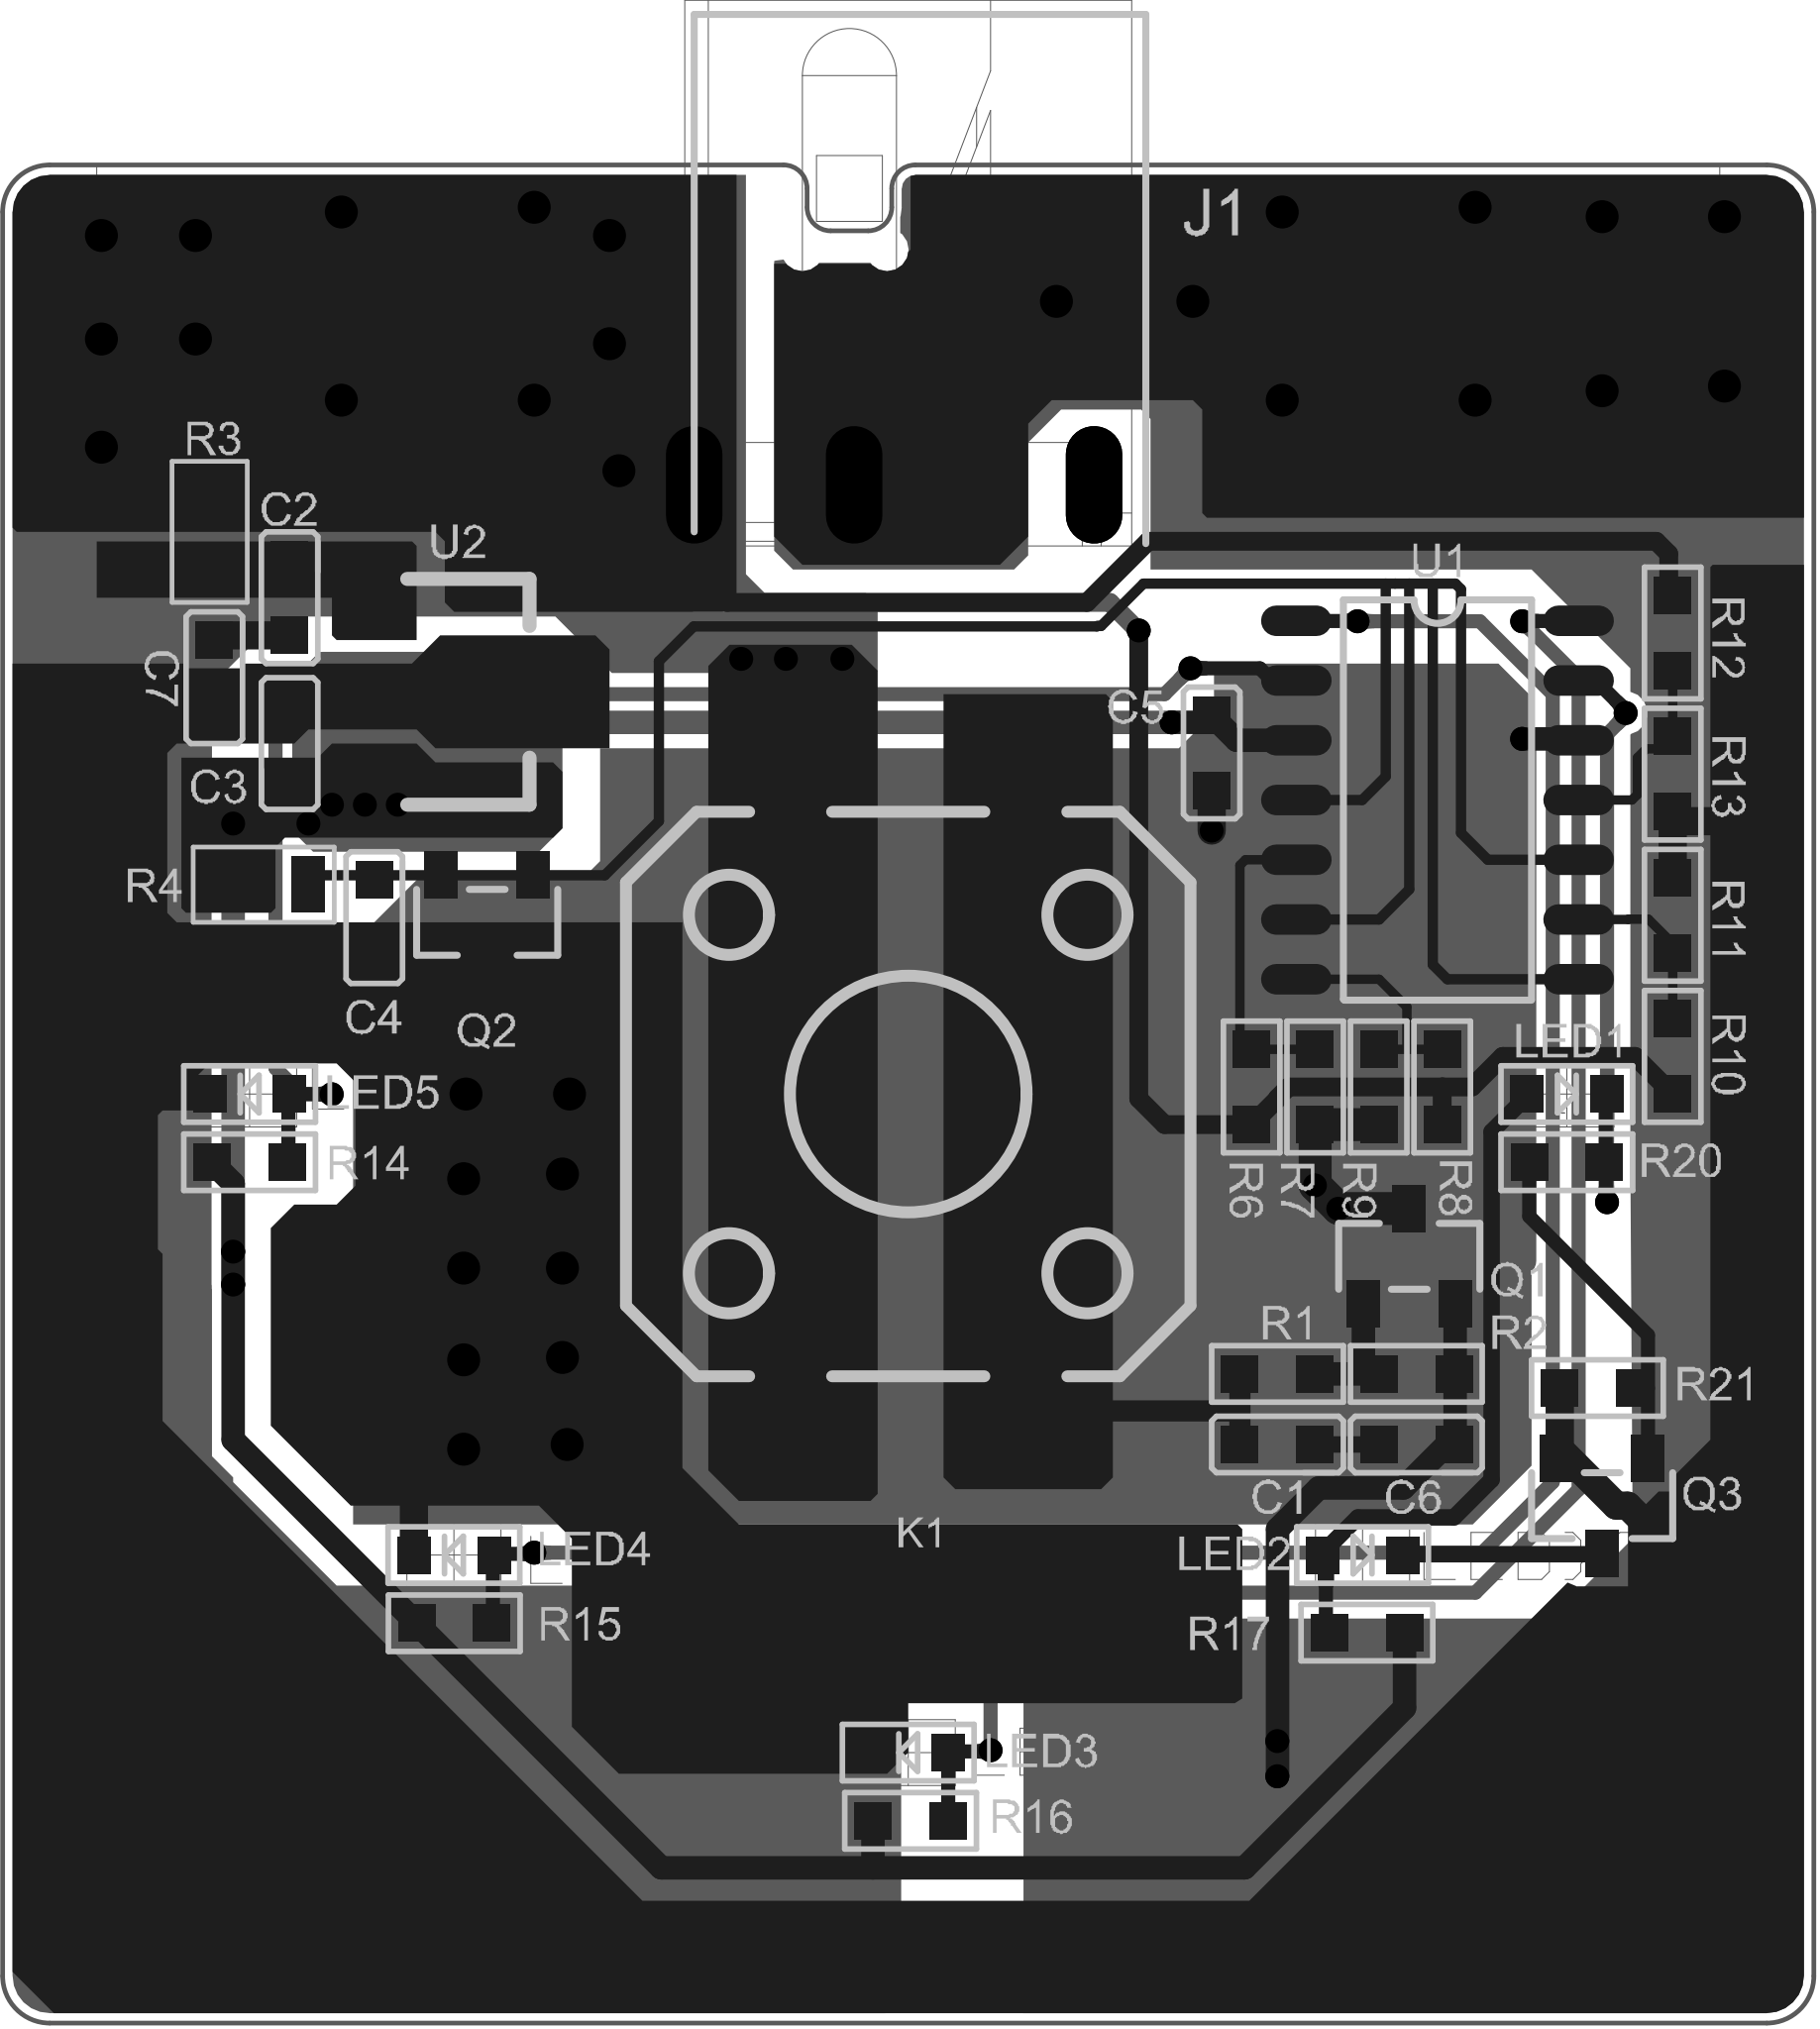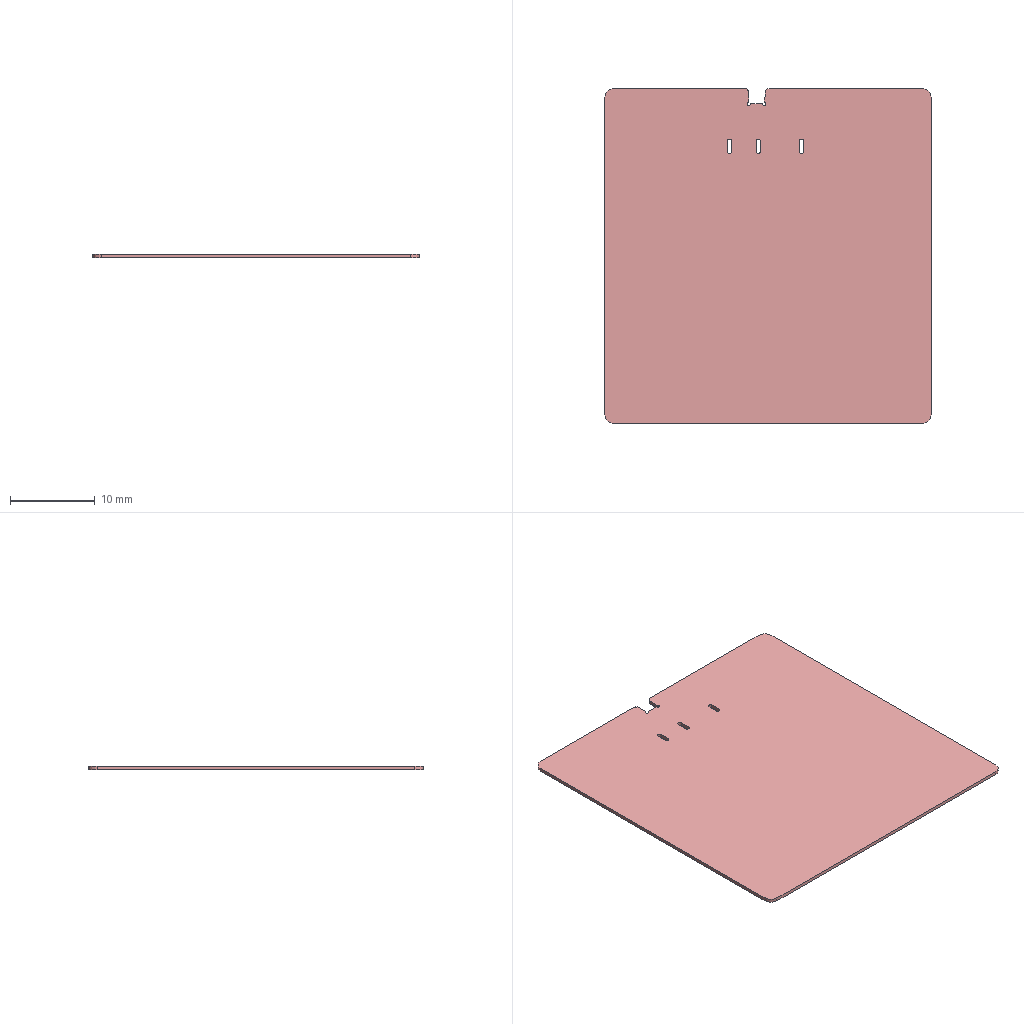Circuit board layout | Altium Designer | box 38.5 x 39.5 x 0.4 mm
Layer stack:
# Altium Designer layer stack of  (unit mm; dielectric type: 0 none, 1 core, 2 prepreg, 3 surface material)
index,name,kind,layer,copper_thickness_mm,dielectric_type,dielectric_thickness_mm,dielectric_material,dielectric_constant
0,Top Paste,other,,,,,,
1,Top Overlay,other,,,,,,
2,Top Solder,dielectric,,,3,0.0102,Solder Resist,3.5
3,Top Layer,copper,Top Layer,0.0356,,,,
4,Dielectric 1,dielectric,,,0,0.32,FR-4,4.8
5,Bottom Layer,copper,Bottom Layer,0.0356,,,,
6,Bottom Solder,dielectric,,,3,0.0102,Solder Resist,3.5
7,Bottom Overlay,other,,,,,,
8,Bottom Paste,other,,,,,,
# drill layer pairs: low layer,high layer
drill_pair,Top Layer,Bottom Layer
Part placement:
Designator,Comment,Layer,Footprint,Center-X(mm),Center-Y(mm),Rotation
U1,LM339,TopLayer,SOP14L,29.5,-13.5,0
K1,SW-PB,TopLayer,SW-SMD_4P-L12.0-W12.0-P5.00-LS15.2,18.25,-19.75,270
J1,DC-044/2.0芯卧插-耐高温260度,TopLayer,DC-044,17.95,-6.8,0
U2,DS8604,TopLayer,SOT-89-3,8.25,-11.2,270
R21,1M,TopLayer,R0603A,32.9,-26,0
R20,100K,TopLayer,R0603A,32.25,-21.2,0
R17,1K,TopLayer,R0603A,28,-31.2,180
R16,1K,TopLayer,R0603A,18.3,-35.2,0
R15,1K,TopLayer,R0603A,8.6,-31,0
R14,1K,TopLayer,R0603A,4.25,-21.2,0
R13,10K 1%,TopLayer,R0603A,34.5,-12.95,90
R12,120K,TopLayer,R0603A,34.5,-9.95,90
R11,10K 1%,TopLayer,R0603A,34.5,-15.95,270
R10,128.4K,TopLayer,R0603A,34.5,-18.95,270
R9,10K 1%,TopLayer,R0603A,28.25,-19.6,90
R8,136.4K,TopLayer,R0603A,29.6,-19.6,270
R7,10K 1%,TopLayer,R0603A,26.9,-19.6,90
R6,145.2K,TopLayer,R0603A,25.55,-19.6,270
R4,2K,TopLayer,R0805A,4.55,-15.3,180
R3,100R,TopLayer,R0805A,3.4,-7.8,90
R2,1M,TopLayer,R0603A,29.05,-25.7,0
R1,3M,TopLayer,R0603A,26.1,-25.7,0
Q3,2N7002,TopLayer,SOT23-3,33,-28.508,180
Q2,TL431_23,TopLayer,SOT23-3,9.3,-16.108,180
Q1,2N7002K,TopLayer,SOT23-3,28.9,-23.192,0
LED5,Green,TopLayer,LED0603A,4.25,-19.75,0
LED4,Green,TopLayer,LED0603A,8.593,-29.55,0
LED3,Green,TopLayer,LED0603A,18.25,-33.75,0
LED2,Green,TopLayer,LED0603A,27.907,-29.55,180
LED1,Green,TopLayer,LED0603A,32.25,-19.75,180
C7,1uF/50V,TopLayer,C0603A,3.5,-10.9,90
C6,1uF/50V,TopLayer,C0603A,29.05,-27.2,0
C5,1uF,TopLayer,C0603A,24.7,-12.5,90
C4,1uF,TopLayer,C0603A,6.9,-16,90
C3,1uF/50V,TopLayer,C0603A,5.1,-12.3,270
C2,1uF/50V,TopLayer,C0603A,5.1,-9.2,90
C1,1uF/50V,TopLayer,C0603A,26.1,-27.2,0
Pad and via stacks:
# Altium Designer via and pad stacks of  (unit mm). Each distinct definition once, with the count of objects using it.
# via: kind,start_layer,end_layer,hole_mm,diameter_mm,mode(0 simple;1 top-mid-bottom;2 full stack),diameter_per_layer,count,example_net
# pad: kind,layer,hole_mm,hole_type(0 round;1 square;2 slot),plating,top_size,top_shape(1 round;2 rect;3 octagon;9 rounded rect),mid_size,bottom_size,mode,footprint,size_per_layer,count,example
pad,Bottom Layer,0,0,plated,4x4,2,4x4,4x4,0,,,4,19
pad,Top Layer,0,0,plated,0.7x0.8,2,0.7x0.8,0.7x0.8,0,LED0603A,,10,LED2.2
pad,Top Layer,0,0,plated,0.8x0.8,2,0.8x0.8,0.8x0.8,0,R0603A,,32,R6.1
pad,Top Layer,0,0,plated,2.64x1.4,2,2.64x1.4,2.64x1.4,0,SW-SMD_4P-L12.0-W12.0-P5.00-LS15.2,,4,K1.1
pad,Top Layer,0,0,plated,0.7x1,2,0.7x1,0.7x1,0,SOT23-3,,9,Q1.1
pad,Top Layer,0,0,plated,0.8x0.8,2,0.8x0.8,0.8x0.8,0,C0603A,,14,C4.2
pad,Top Layer,0,0,plated,1x1,1,1x1,1x1,0,,,2,21
pad,Top Layer,0,2,plated,0.65x1.5,1,0.65x1.5,0.65x1.5,0,SOP14L,,14,U1.10
pad,Top Layer,0,0,plated,0.7x1.2,2,0.7x1.2,0.7x1.2,0,R0805A,,4,R4.2
pad,Top Layer,0,2,plated,1.5x0.65,2,1.5x0.65,1.5x0.65,0,SOT-89-3,,3,U2.1
pad,Top Layer,0,2,plated,2x3.8,1,2x3.8,2x3.8,0,SOT-89-3,,1,U2.2
pad,Multi-Layer,0.5,2,plated,2.5x1.2,1,2.5x1.2,2.5x1.2,0,DC-044,,3,J1.1
via,Top Layer,Bottom Layer,0.3048,0.508,0,,26,P+
via,Top Layer,Bottom Layer,0.5,0.7,0,,32,GND
Copper pours:
name,layer,net,type(0 solid;1 hatched;2 none)
NONET_L02_P-001,Bottom Layer,GND,0
NONET_L02_P-001,Bottom Layer,P-,0
NONET_L02_P-001,Bottom Layer,5V,0
NONET_L02_P-001,Bottom Layer,P+,0
NONET_L02_P-001,Top Layer,GND,0
NONET_L02_P-001,Top Layer,P+,0
NONET_L02_P-001,Top Layer,NetC1_1,0
NONET_L02_P-001,Top Layer,P-,0
NONET_L02_P-001,Top Layer,NetC2_2,0
NONET_L02_P-001,Top Layer,5V,0
NONET_L02_P-001,Top Layer,P+,0
Design rules, without the lines most boards share:
# Altium Designer design rules of  (exported by Altium Designer, unit mm)
# columns: name | kind | enabled | priority | scope1 | scope2 | descriptor | typed fields (field=value)
Schematic Supply Nets_4 | 41 | enabled | 1 | InNet('GND') | All | Supply Net(s)(InNet('GND')) |
Schematic Supply Nets_3 | 41 | enabled | 2 | InNet('2.5V') | All | Supply Net(s)(InNet('2.5V')) |
Schematic Supply Nets | 41 | enabled | 3 | InNet('5V') | All | Supply Net(s)(InNet('5V')) |
NetAntennae | 56 | enabled | 1 | All | All | Net Antennae (Tolerance=0mm) (All) |
SilkToSilkClearance | 55 | enabled | 1 | All | All | Silk to Silk (Clearance=0mm) (All),(All) |
SilkToSolderMaskClearance | 54 | enabled | 1 | IsPad | All | Silk To Solder Mask (Clearance=0mm) (IsPad),(All) |
MinimumSolderMaskSliver | 53 | enabled | 1 | All | All | Minimum Solder Mask Sliver (Gap=0.01mm) (All),(All) |
HoleToHoleClearance | 52 | enabled | 1 | All | All | Hole To Hole Clearance (Gap=0.254mm) (All),(All) | gap=0.254
DiffPairsRouting | 51 | enabled | 1 | All | All | Differential Pairs Uncoupled Length using the Gap Constraints (Min=0.254mm) (Max=0.254mm) (Prefered=0.254mm)  and Width Constraints (Min=0.381mm) (Max=0.381mm) (Prefered=0.381mm) (All) |
HoleSize | 42 | enabled | 1 | All | All | Hole Size Constraint (Min=0.025mm) (Max=2.54mm) (All) |
Height | 50 | enabled | 1 | All | All | Height Constraint (Min=0mm) (Max=25.4mm) (Prefered=12.7mm) (All) | min_height=0 max_height=25.4
ComponentClearance | 24 | enabled | 1 | All | All | Component Clearance Constraint ( Horizontal Gap = 0.254mm, Vertical Gap = 0.254mm ) (All),(All)  | gap=0.254
SolderMaskExpansion | 13 | enabled | 1 | All | All | Solder Mask Expansion (Expansion =0.102mm) (All) | expansion=0.1016
PasteMaskExpansion | 14 | enabled | 1 | All | All | Paste Mask Expansion (Expansion =0mm) (All) | expansion=0
RoutingVias | 11 | enabled | 1 | All | All | Routing Via (MinHoleWidth=0.711mm) (MaxHoleWidth=0.711mm) (PreferredHoleWidth=0.711mm) (MinWidth=1.27mm) (MaxWidth=1.27mm) (PreferedWidth=1.27mm) (All) | via_min_hole=0.7112 via_max_hole=0.7112 via_preferred_diameter=1.27 via_preferred_hole=0.7112
RoutingCorners | 10 | enabled | 1 | All | All | Routing Corners (Style=45-Degree) (Min Setback=2.54mm) (Max Setback=2.54mm) (All) |
Width | 2 | enabled | 1 | All | All | Width Constraint (Min=0.2mm) (Max=1mm) (Preferred=0.3mm) (All) |
PolygonConnect | 20 | enabled | 1 | All | All | Polygon Connect Rule(Direct Connect )(Conductor Width=0.254mm) (Relief Angle=90 Angle) (Entries=4) (Air Gap Width=0.254mm) (All),(All) | connect_style(0=relief,1=direct,2=none)=1 relief_conductor_width=0.254 relief_entries=4
PlaneClearance | 12 | enabled | 1 | All | All | Power Plane Clearance (Clearance =0.508mm) (All) | clearance=0.508
PlaneConnect | 6 | enabled | 1 | All | All | Power Plane Connect Rule(Relief Connect )(Expansion=0.508mm) (Conductor Width=0.254mm) (Air Gap=0.254mm) (Entries=4) (All) | relief_conductor_width=0.254 relief_entries=4 relief_expansion=0.508
Clearance | 0 | enabled | 1 | All | All | Clearance Constraint (Gap=0.2mm) (All),(All) | gap=0.2